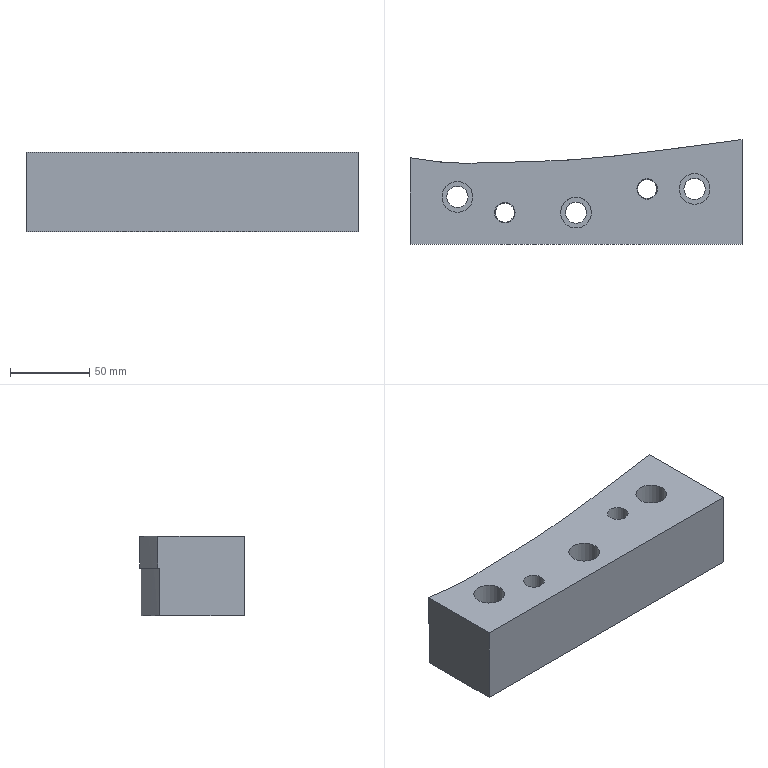Part | NX | features solid 2 | 1 solid | 23 faces | box 210 x 66.209 x 50 mm | volume 539295 mm3 | plane 11 | cylinder 10 | spline 2 | commonest cylinder face diameters 13.5 x3 19.5 x3 12 x2 13 x2
STEP:
#1=CARTESIAN_POINT('',(95.,106.209,-20.));
#2=VERTEX_POINT('',#1);
#3=CARTESIAN_POINT('',(95.,106.209,0.));
#4=VERTEX_POINT('',#3);
#5=CARTESIAN_POINT('',(95.,106.209,-10.));
#6=DIRECTION('',(0.,0.,-1.));
#7=VECTOR('',#6,1000.);
#8=LINE('',#5,#7);
#9=EDGE_CURVE('',#2,#4,#8,.F.);
#10=ORIENTED_EDGE('',*,*,#9,.F.);
#11=CARTESIAN_POINT('',(-115.,94.682,-20.));
#12=VERTEX_POINT('',#11);
#13=CARTESIAN_POINT('',(-190.231,-121.49,-20.));
#14=CARTESIAN_POINT('',(-188.654,-121.152,-20.));
#15=CARTESIAN_POINT('',(-185.47,-120.627,-20.));
#16=CARTESIAN_POINT('',(-180.656,-120.141,-20.));
#17=CARTESIAN_POINT('',(-175.882,-119.326,-20.));
#18=CARTESIAN_POINT('',(-169.679,-117.528,-20.));
#19=CARTESIAN_POINT('',(-162.185,-114.539,-20.));
#20=CARTESIAN_POINT('',(-153.086,-111.254,-20.));
#21=CARTESIAN_POINT('',(-144.031,-107.845,-20.));
#22=CARTESIAN_POINT('',(-136.465,-105.061,-20.));
#23=CARTESIAN_POINT('',(-130.418,-102.814,-20.));
#24=CARTESIAN_POINT('',(-125.812,-101.329,-20.));
#25=CARTESIAN_POINT('',(-121.306,-99.566,-20.));
#26=CARTESIAN_POINT('',(-116.876,-97.626,-20.));
#27=CARTESIAN_POINT('',(-112.335,-95.923,-20.));
#28=CARTESIAN_POINT('',(-107.564,-95.05,-20.));
#29=CARTESIAN_POINT('',(-102.756,-94.525,-20.));
#30=CARTESIAN_POINT('',(-96.349,-93.771,-20.));
#31=CARTESIAN_POINT('',(-89.902,-93.468,-20.));
#32=CARTESIAN_POINT('',(-83.452,-93.448,-20.));
#33=CARTESIAN_POINT('',(-77.002,-93.469,-20.));
#34=CARTESIAN_POINT('',(-68.939,-93.411,-20.));
#35=CARTESIAN_POINT('',(-56.04,-93.3,-20.));
#36=CARTESIAN_POINT('',(-33.465,-93.184,-20.));
#37=CARTESIAN_POINT('',(-7.666,-93.074,-20.));
#38=CARTESIAN_POINT('',(14.907,-92.653,-20.));
#39=CARTESIAN_POINT('',(27.794,-92.068,-20.));
#40=CARTESIAN_POINT('',(40.668,-91.245,-20.));
#41=CARTESIAN_POINT('',(51.917,-90.291,-20.));
#42=CARTESIAN_POINT('',(61.528,-89.174,-20.));
#43=CARTESIAN_POINT('',(67.939,-88.466,-20.));
#44=CARTESIAN_POINT('',(79.125,-86.95,-20.));
#45=CARTESIAN_POINT('',(95.161,-85.253,-20.));
#46=CARTESIAN_POINT('',(114.404,-83.21,-20.));
#47=CARTESIAN_POINT('',(133.568,-80.524,-20.));
#48=CARTESIAN_POINT('',(152.734,-77.861,-20.));
#49=CARTESIAN_POINT('',(171.916,-75.326,-20.));
#50=CARTESIAN_POINT('',(191.055,-72.413,-20.));
#51=CARTESIAN_POINT('',(207.17,-71.468,-20.));
#52=CARTESIAN_POINT('',(219.951,-69.697,-20.));
#53=CARTESIAN_POINT('',(232.724,-67.899,-20.));
#54=CARTESIAN_POINT('',(248.708,-65.766,-20.));
#55=CARTESIAN_POINT('',(267.87,-63.074,-20.));
#56=CARTESIAN_POINT('',(287.038,-60.44,-20.));
#57=CARTESIAN_POINT('',(301.448,-58.682,-20.));
#58=CARTESIAN_POINT('',(310.976,-56.987,-20.));
#59=CARTESIAN_POINT('',(314.916,-56.135,-20.));
#60=CARTESIAN_POINT('',(318.052,-55.382,-20.));
#61=CARTESIAN_POINT('',(320.39,-54.76,-20.));
#62=CARTESIAN_POINT('',(322.686,-53.981,-20.));
#63=CARTESIAN_POINT('',(325.595,-52.578,-20.));
#64=CARTESIAN_POINT('',(328.769,-50.098,-20.));
#65=CARTESIAN_POINT('',(332.247,-46.69,-20.));
#66=CARTESIAN_POINT('',(335.795,-43.406,-20.));
#67=CARTESIAN_POINT('',(343.661,-37.758,-20.));
#68=CARTESIAN_POINT('',(355.164,-28.914,-20.));
#69=CARTESIAN_POINT('',(370.422,-17.018,-20.));
#70=CARTESIAN_POINT('',(383.264,-7.249,-20.));
#71=CARTESIAN_POINT('',(392.416,-0.6713,-20.));
#72=CARTESIAN_POINT('',(396.953,2.733,-20.));
#73=CARTESIAN_POINT('',(398.886,5.372,-20.));
#74=CARTESIAN_POINT('',(399.725,7.654,-20.));
#75=CARTESIAN_POINT('',(399.76,10.078,-20.));
#76=CARTESIAN_POINT('',(399.483,13.317,-20.));
#77=CARTESIAN_POINT('',(399.712,17.34,-20.));
#78=CARTESIAN_POINT('',(399.612,22.179,-20.));
#79=CARTESIAN_POINT('',(399.633,31.854,-20.));
#80=CARTESIAN_POINT('',(399.593,46.366,-20.));
#81=CARTESIAN_POINT('',(399.637,62.491,-20.));
#82=CARTESIAN_POINT('',(399.588,73.779,-20.));
#83=CARTESIAN_POINT('',(399.652,79.422,-20.));
#84=CARTESIAN_POINT('',(399.59,82.647,-20.));
#85=CARTESIAN_POINT('',(399.564,85.065,-20.));
#86=CARTESIAN_POINT('',(399.725,87.486,-20.));
#87=CARTESIAN_POINT('',(399.756,89.902,-20.));
#88=CARTESIAN_POINT('',(399.247,92.301,-20.));
#89=CARTESIAN_POINT('',(397.362,95.008,-20.));
#90=CARTESIAN_POINT('',(393.635,96.774,-20.));
#91=CARTESIAN_POINT('',(389.279,98.826,-20.));
#92=CARTESIAN_POINT('',(384.732,100.498,-20.));
#93=CARTESIAN_POINT('',(378.765,102.95,-20.));
#94=CARTESIAN_POINT('',(362.589,110.229,-20.));
#95=CARTESIAN_POINT('',(344.928,118.135,-20.));
#96=CARTESIAN_POINT('',(327.281,126.072,-20.));
#97=CARTESIAN_POINT('',(319.932,129.381,-20.));
#98=CARTESIAN_POINT('',(314.075,132.102,-20.));
#99=CARTESIAN_POINT('',(309.387,133.376,-20.));
#100=CARTESIAN_POINT('',(304.547,133.785,-20.));
#101=CARTESIAN_POINT('',(299.716,133.401,-20.));
#102=CARTESIAN_POINT('',(294.929,132.704,-20.));
#103=CARTESIAN_POINT('',(288.543,131.8,-20.));
#104=CARTESIAN_POINT('',(277.364,130.241,-20.));
#105=CARTESIAN_POINT('',(242.2,125.552,-20.));
#106=CARTESIAN_POINT('',(184.637,118.048,-20.));
#107=CARTESIAN_POINT('',(120.701,109.541,-20.));
#108=CARTESIAN_POINT('',(69.531,102.902,-20.));
#109=CARTESIAN_POINT('',(40.777,98.94,-20.));
#110=CARTESIAN_POINT('',(21.566,96.615,-20.));
#111=CARTESIAN_POINT('',(8.743,95.212,-20.));
#112=CARTESIAN_POINT('',(-7.301,93.575,-20.));
#113=CARTESIAN_POINT('',(-26.625,92.505,-20.));
#114=CARTESIAN_POINT('',(-45.971,92.017,-20.));
#115=CARTESIAN_POINT('',(-62.09,91.675,-20.));
#116=CARTESIAN_POINT('',(-74.987,91.256,-20.));
#117=CARTESIAN_POINT('',(-84.664,91.165,-20.));
#118=CARTESIAN_POINT('',(-94.319,91.781,-20.));
#119=CARTESIAN_POINT('',(-103.929,92.966,-20.));
#120=CARTESIAN_POINT('',(-113.495,94.403,-20.));
#121=CARTESIAN_POINT('',(-119.856,95.492,-20.));
#122=CARTESIAN_POINT('',(-122.997,96.222,-20.));
#123=B_SPLINE_CURVE_WITH_KNOTS('',3,(#13,#14,#15,#16,#17,#18,#19,#20,#21,#22,#23,#24,#25,#26,#27,#28,#29,#30,#31,#32,#33,#34,#35,#36,#37,#38,#39,#40,#41,#42,#43,#44,#45,#46,#47,#48,#49,#50,#51,#52,#53,#54,#55,#56,#57,#58,#59,#60,#61,#62,#63,#64,#65,#66,#67,#68,#69,#70,#71,#72,#73,#74,#75,#76,#77,#78,#79,#80,#81,#82,#83,#84,#85,#86,#87,#88,#89,#90,#91,#92,#93,#94,#95,#96,#97,#98,#99,#100,#101,#102,#103,#104,#105,#106,#107,#108,#109,#110,#111,#112,#113,#114,#115,#116,#117,#118,#119,#120,#121,#122),.UNSPECIFIED.,.F.,.F.,(4,1,1,1,1,1,1,1,1,1,1,1,1,1,1,1,1,1,1,1,1,1,1,1,1,1,1,1,1,1,1,1,1,1,1,1,1,1,1,1,1,1,1,1,1,1,1,1,1,1,1,1,1,1,1,1,1,1,1,1,1,1,1,1,1,1,1,1,1,1,1,1,1,1,1,1,1,1,1,1,1,1,1,1,1,1,1,1,1,1,1,1,1,1,1,1,1,1,1,1,1,1,1,1,1,1,1,4),(0.4704,0.4724,0.4745,0.4766,0.4786,0.4828,0.4869,0.491,0.4952,0.4972,0.4993,0.5014,0.5035,0.5055,0.5076,0.5097,0.5117,0.5159,0.5179,0.52,0.5241,0.5283,0.5366,0.5531,0.5614,0.5655,0.5697,0.5779,0.58,0.5821,0.5862,0.5945,0.6028,0.611,0.6193,0.6276,0.6359,0.6441,0.6483,0.6524,0.6607,0.669,0.6772,0.6855,0.6876,0.6897,0.6907,0.6917,0.6928,0.6938,0.6959,0.6979,0.7,0.7021,0.7103,0.7186,0.7269,0.731,0.7331,0.7341,0.7352,0.7362,0.7372,0.7393,0.7414,0.7435,0.7517,0.76,0.7641,0.7662,0.7672,0.7683,0.7693,0.7703,0.7714,0.7724,0.7745,0.7766,0.7786,0.7807,0.7848,0.8014,0.8055,0.8097,0.8117,0.8138,0.8159,0.8179,0.82,0.8221,0.8262,0.8345,0.8676,0.9007,0.9172,0.9338,0.9379,0.9421,0.9503,0.9586,0.9669,0.9752,0.9793,0.9834,0.9876,0.9917,0.9959,1.),.UNSPECIFIED.);
#124=EDGE_CURVE('',#2,#12,#123,.T.);
#125=ORIENTED_EDGE('',*,*,#124,.T.);
#126=CARTESIAN_POINT('',(-115.,94.682,0.));
#127=VERTEX_POINT('',#126);
#128=CARTESIAN_POINT('',(-115.,94.682,-35.));
#129=DIRECTION('',(0.,0.,-1.));
#130=VECTOR('',#129,1000.);
#131=LINE('',#128,#130);
#132=EDGE_CURVE('',#12,#127,#131,.F.);
#133=ORIENTED_EDGE('',*,*,#132,.T.);
#134=CARTESIAN_POINT('',(-115.,94.682,0.));
#135=CARTESIAN_POINT('',(-110.608,93.956,0.));
#136=CARTESIAN_POINT('',(-101.827,92.632,0.));
#137=CARTESIAN_POINT('',(-84.275,90.758,0.));
#138=CARTESIAN_POINT('',(-62.384,91.781,0.));
#139=CARTESIAN_POINT('',(-36.103,92.158,0.));
#140=CARTESIAN_POINT('',(-9.834,93.269,0.));
#141=CARTESIAN_POINT('',(16.416,95.966,0.));
#142=CARTESIAN_POINT('',(42.64,99.193,0.));
#143=CARTESIAN_POINT('',(68.808,102.78,0.));
#144=CARTESIAN_POINT('',(86.269,105.068,0.));
#145=CARTESIAN_POINT('',(95.,106.209,0.));
#146=B_SPLINE_CURVE_WITH_KNOTS('',3,(#134,#135,#136,#137,#138,#139,#140,#141,#142,#143,#144,#145),.UNSPECIFIED.,.F.,.F.,(4,1,1,1,1,1,1,1,1,4),(0.,0.01314,0.02628,0.05257,0.07885,0.1051,0.1314,0.1577,0.184,0.2103),.UNSPECIFIED.);
#147=EDGE_CURVE('',#127,#4,#146,.T.);
#148=ORIENTED_EDGE('',*,*,#147,.T.);
#149=EDGE_LOOP('',(#10,#125,#133,#148));
#150=FACE_BOUND('',#149,.T.);
#151=CARTESIAN_POINT('',(95.,106.209,0.));
#152=CARTESIAN_POINT('',(95.,106.209,-20.));
#153=CARTESIAN_POINT('',(86.281,105.069,0.));
#154=CARTESIAN_POINT('',(86.281,105.069,-20.));
#155=CARTESIAN_POINT('',(68.844,102.785,0.));
#156=CARTESIAN_POINT('',(68.844,102.785,-20.));
#157=CARTESIAN_POINT('',(42.708,99.202,0.));
#158=CARTESIAN_POINT('',(42.708,99.202,-20.));
#159=CARTESIAN_POINT('',(16.527,95.979,0.));
#160=CARTESIAN_POINT('',(16.527,95.979,-20.));
#161=CARTESIAN_POINT('',(-9.721,93.276,0.));
#162=CARTESIAN_POINT('',(-9.721,93.276,-20.));
#163=CARTESIAN_POINT('',(-36.089,92.158,0.));
#164=CARTESIAN_POINT('',(-36.089,92.158,-20.));
#165=CARTESIAN_POINT('',(-62.452,91.777,0.));
#166=CARTESIAN_POINT('',(-62.452,91.777,-20.));
#167=CARTESIAN_POINT('',(-84.459,90.762,0.));
#168=CARTESIAN_POINT('',(-84.459,90.762,-20.));
#169=CARTESIAN_POINT('',(-101.968,92.654,0.));
#170=CARTESIAN_POINT('',(-101.968,92.654,-20.));
#171=CARTESIAN_POINT('',(-110.662,93.965,0.));
#172=CARTESIAN_POINT('',(-110.662,93.965,-20.));
#173=CARTESIAN_POINT('',(-115.,94.682,0.));
#174=CARTESIAN_POINT('',(-115.,94.682,-20.));
#175=B_SPLINE_SURFACE_WITH_KNOTS('',3,1,((#151,#152),(#153,#154),(#155,#156),(#157,#158),(#159,#160),(#161,#162),(#163,#164),(#165,#166),(#167,#168),(#169,#170),(#171,#172),(#173,#174)),.SURF_OF_LINEAR_EXTRUSION.,.F.,.F.,.F.,(4,1,1,1,1,1,1,1,1,4),(2,2),(0.9063,0.9175,0.9288,0.9401,0.9514,0.9627,0.974,0.9852,0.9909,0.9965),(0.,1.),.UNSPECIFIED.);
#176=ADVANCED_FACE('',(#150),#175,.F.);
#177=CARTESIAN_POINT('',(95.,105.2,-20.));
#178=VERTEX_POINT('',#177);
#179=CARTESIAN_POINT('',(95.,83.097,-20.));
#180=DIRECTION('',(0.,-1.,0.));
#181=VECTOR('',#180,1000.);
#182=LINE('',#179,#181);
#183=EDGE_CURVE('',#2,#178,#182,.T.);
#184=ORIENTED_EDGE('',*,*,#183,.F.);
#185=ORIENTED_EDGE('',*,*,#9,.T.);
#186=CARTESIAN_POINT('',(95.,40.,0.));
#187=VERTEX_POINT('',#186);
#188=CARTESIAN_POINT('',(95.,-222.,0.));
#189=DIRECTION('',(0.,-1.,0.));
#190=VECTOR('',#189,1000.);
#191=LINE('',#188,#190);
#192=EDGE_CURVE('',#4,#187,#191,.T.);
#193=ORIENTED_EDGE('',*,*,#192,.T.);
#194=CARTESIAN_POINT('',(95.,40.,-50.));
#195=VERTEX_POINT('',#194);
#196=CARTESIAN_POINT('',(95.,40.,0.));
#197=DIRECTION('',(0.,0.,-1.));
#198=VECTOR('',#197,1000.);
#199=LINE('',#196,#198);
#200=EDGE_CURVE('',#187,#195,#199,.T.);
#201=ORIENTED_EDGE('',*,*,#200,.T.);
#202=CARTESIAN_POINT('',(95.,105.2,-50.));
#203=VERTEX_POINT('',#202);
#204=CARTESIAN_POINT('',(95.,35.09,-50.));
#205=DIRECTION('',(0.,1.,0.));
#206=VECTOR('',#205,1000.);
#207=LINE('',#204,#206);
#208=EDGE_CURVE('',#195,#203,#207,.T.);
#209=ORIENTED_EDGE('',*,*,#208,.T.);
#210=CARTESIAN_POINT('',(95.,105.2,-60.));
#211=DIRECTION('',(0.,0.,-1.));
#212=VECTOR('',#211,1000.);
#213=LINE('',#210,#212);
#214=EDGE_CURVE('',#178,#203,#213,.T.);
#215=ORIENTED_EDGE('',*,*,#214,.F.);
#216=EDGE_LOOP('',(#184,#185,#193,#201,#209,#215));
#217=FACE_BOUND('',#216,.T.);
#218=CARTESIAN_POINT('',(95.,83.097,-25.));
#219=DIRECTION('',(1.,0.,0.));
#220=DIRECTION('',(0.,0.,-1.));
#221=AXIS2_PLACEMENT_3D('',#218,#219,#220);
#222=PLANE('',#221);
#223=ADVANCED_FACE('',(#217),#222,.T.);
#224=ORIENTED_EDGE('',*,*,#132,.F.);
#225=CARTESIAN_POINT('',(-115.,93.668,-20.));
#226=VERTEX_POINT('',#225);
#227=CARTESIAN_POINT('',(-115.,30.,-20.));
#228=DIRECTION('',(0.,-1.,0.));
#229=VECTOR('',#228,1000.);
#230=LINE('',#227,#229);
#231=EDGE_CURVE('',#12,#226,#230,.T.);
#232=ORIENTED_EDGE('',*,*,#231,.T.);
#233=CARTESIAN_POINT('',(-115.,93.668,-50.));
#234=VERTEX_POINT('',#233);
#235=CARTESIAN_POINT('',(-115.,93.668,-60.));
#236=DIRECTION('',(0.,0.,-1.));
#237=VECTOR('',#236,1000.);
#238=LINE('',#235,#237);
#239=EDGE_CURVE('',#226,#234,#238,.T.);
#240=ORIENTED_EDGE('',*,*,#239,.T.);
#241=CARTESIAN_POINT('',(-115.,40.,-50.));
#242=VERTEX_POINT('',#241);
#243=CARTESIAN_POINT('',(-115.,35.09,-50.));
#244=DIRECTION('',(0.,1.,0.));
#245=VECTOR('',#244,1000.);
#246=LINE('',#243,#245);
#247=EDGE_CURVE('',#242,#234,#246,.T.);
#248=ORIENTED_EDGE('',*,*,#247,.F.);
#249=CARTESIAN_POINT('',(-115.,40.,0.));
#250=VERTEX_POINT('',#249);
#251=CARTESIAN_POINT('',(-115.,40.,0.));
#252=DIRECTION('',(0.,0.,1.));
#253=VECTOR('',#252,1000.);
#254=LINE('',#251,#253);
#255=EDGE_CURVE('',#242,#250,#254,.T.);
#256=ORIENTED_EDGE('',*,*,#255,.T.);
#257=CARTESIAN_POINT('',(-115.,-222.,0.));
#258=DIRECTION('',(0.,-1.,0.));
#259=VECTOR('',#258,1000.);
#260=LINE('',#257,#259);
#261=EDGE_CURVE('',#127,#250,#260,.T.);
#262=ORIENTED_EDGE('',*,*,#261,.F.);
#263=EDGE_LOOP('',(#224,#232,#240,#248,#256,#262));
#264=FACE_BOUND('',#263,.T.);
#265=CARTESIAN_POINT('',(-115.,30.,0.));
#266=DIRECTION('',(1.,0.,0.));
#267=DIRECTION('',(0.,0.,-1.));
#268=AXIS2_PLACEMENT_3D('',#265,#266,#267);
#269=PLANE('',#268);
#270=ADVANCED_FACE('',(#264),#269,.F.);
#271=ORIENTED_EDGE('',*,*,#200,.F.);
#272=CARTESIAN_POINT('',(-470.381,40.,0.));
#273=DIRECTION('',(1.,0.,0.));
#274=VECTOR('',#273,1000.);
#275=LINE('',#272,#274);
#276=EDGE_CURVE('',#250,#187,#275,.T.);
#277=ORIENTED_EDGE('',*,*,#276,.F.);
#278=ORIENTED_EDGE('',*,*,#255,.F.);
#279=CARTESIAN_POINT('',(-415.478,40.,-50.));
#280=DIRECTION('',(-1.,0.,0.));
#281=VECTOR('',#280,1000.);
#282=LINE('',#279,#281);
#283=EDGE_CURVE('',#195,#242,#282,.T.);
#284=ORIENTED_EDGE('',*,*,#283,.F.);
#285=EDGE_LOOP('',(#271,#277,#278,#284));
#286=FACE_BOUND('',#285,.T.);
#287=CARTESIAN_POINT('',(180.,40.,0.));
#288=DIRECTION('',(0.,1.,0.));
#289=DIRECTION('',(0.,0.,1.));
#290=AXIS2_PLACEMENT_3D('',#287,#288,#289);
#291=PLANE('',#290);
#292=ADVANCED_FACE('',(#286),#291,.F.);
#293=CARTESIAN_POINT('',(28.5,75.,0.));
#294=VERTEX_POINT('',#293);
#295=CARTESIAN_POINT('',(35.,75.,0.));
#296=DIRECTION('',(0.,0.,-1.));
#297=DIRECTION('',(-1.,0.,0.));
#298=AXIS2_PLACEMENT_3D('',#295,#296,#297);
#299=CIRCLE('',#298,6.5);
#300=EDGE_CURVE('',#294,#294,#299,.T.);
#301=ORIENTED_EDGE('',*,*,#300,.T.);
#302=EDGE_LOOP('',(#301));
#303=FACE_BOUND('',#302,.T.);
#304=CARTESIAN_POINT('',(-61.5,60.,0.));
#305=VERTEX_POINT('',#304);
#306=CARTESIAN_POINT('',(-55.,60.,0.));
#307=DIRECTION('',(0.,0.,-1.));
#308=DIRECTION('',(-1.,0.,0.));
#309=AXIS2_PLACEMENT_3D('',#306,#307,#308);
#310=CIRCLE('',#309,6.5);
#311=EDGE_CURVE('',#305,#305,#310,.T.);
#312=ORIENTED_EDGE('',*,*,#311,.T.);
#313=EDGE_LOOP('',(#312));
#314=FACE_BOUND('',#313,.T.);
#315=CARTESIAN_POINT('',(-19.75,60.,0.));
#316=VERTEX_POINT('',#315);
#317=CARTESIAN_POINT('',(-10.,60.,0.));
#318=DIRECTION('',(0.,0.,-1.));
#319=DIRECTION('',(-1.,0.,0.));
#320=AXIS2_PLACEMENT_3D('',#317,#318,#319);
#321=CIRCLE('',#320,9.75);
#322=EDGE_CURVE('',#316,#316,#321,.T.);
#323=ORIENTED_EDGE('',*,*,#322,.T.);
#324=EDGE_LOOP('',(#323));
#325=FACE_BOUND('',#324,.T.);
#326=CARTESIAN_POINT('',(55.25,75.,0.));
#327=VERTEX_POINT('',#326);
#328=CARTESIAN_POINT('',(65.,75.,0.));
#329=DIRECTION('',(0.,0.,-1.));
#330=DIRECTION('',(-1.,0.,0.));
#331=AXIS2_PLACEMENT_3D('',#328,#329,#330);
#332=CIRCLE('',#331,9.75);
#333=EDGE_CURVE('',#327,#327,#332,.T.);
#334=ORIENTED_EDGE('',*,*,#333,.T.);
#335=EDGE_LOOP('',(#334));
#336=FACE_BOUND('',#335,.T.);
#337=CARTESIAN_POINT('',(-94.75,70.,0.));
#338=VERTEX_POINT('',#337);
#339=CARTESIAN_POINT('',(-85.,70.,0.));
#340=DIRECTION('',(0.,0.,-1.));
#341=DIRECTION('',(-1.,0.,0.));
#342=AXIS2_PLACEMENT_3D('',#339,#340,#341);
#343=CIRCLE('',#342,9.75);
#344=EDGE_CURVE('',#338,#338,#343,.T.);
#345=ORIENTED_EDGE('',*,*,#344,.T.);
#346=EDGE_LOOP('',(#345));
#347=FACE_BOUND('',#346,.T.);
#348=ORIENTED_EDGE('',*,*,#192,.F.);
#349=ORIENTED_EDGE('',*,*,#147,.F.);
#350=ORIENTED_EDGE('',*,*,#261,.T.);
#351=ORIENTED_EDGE('',*,*,#276,.T.);
#352=EDGE_LOOP('',(#348,#349,#350,#351));
#353=FACE_BOUND('',#352,.T.);
#354=CARTESIAN_POINT('',(-470.381,-222.,0.));
#355=DIRECTION('',(0.,0.,-1.));
#356=DIRECTION('',(-1.,0.,0.));
#357=AXIS2_PLACEMENT_3D('',#354,#355,#356);
#358=PLANE('',#357);
#359=ADVANCED_FACE('',(#303,#314,#325,#336,#347,#353),#358,.F.);
#360=CARTESIAN_POINT('',(41.,75.,-50.));
#361=VERTEX_POINT('',#360);
#362=CARTESIAN_POINT('',(35.,75.,-50.));
#363=DIRECTION('',(0.,0.,1.));
#364=DIRECTION('',(1.,0.,0.));
#365=AXIS2_PLACEMENT_3D('',#362,#363,#364);
#366=CIRCLE('',#365,6.);
#367=EDGE_CURVE('',#361,#361,#366,.T.);
#368=ORIENTED_EDGE('',*,*,#367,.T.);
#369=EDGE_LOOP('',(#368));
#370=FACE_BOUND('',#369,.T.);
#371=CARTESIAN_POINT('',(-49.,60.,-50.));
#372=VERTEX_POINT('',#371);
#373=CARTESIAN_POINT('',(-55.,60.,-50.));
#374=DIRECTION('',(0.,0.,1.));
#375=DIRECTION('',(1.,0.,0.));
#376=AXIS2_PLACEMENT_3D('',#373,#374,#375);
#377=CIRCLE('',#376,6.);
#378=EDGE_CURVE('',#372,#372,#377,.T.);
#379=ORIENTED_EDGE('',*,*,#378,.T.);
#380=EDGE_LOOP('',(#379));
#381=FACE_BOUND('',#380,.T.);
#382=CARTESIAN_POINT('',(-3.25,60.,-50.));
#383=VERTEX_POINT('',#382);
#384=CARTESIAN_POINT('',(-10.,60.,-50.));
#385=DIRECTION('',(0.,0.,1.));
#386=DIRECTION('',(1.,0.,0.));
#387=AXIS2_PLACEMENT_3D('',#384,#385,#386);
#388=CIRCLE('',#387,6.75);
#389=EDGE_CURVE('',#383,#383,#388,.T.);
#390=ORIENTED_EDGE('',*,*,#389,.T.);
#391=EDGE_LOOP('',(#390));
#392=FACE_BOUND('',#391,.T.);
#393=CARTESIAN_POINT('',(71.75,75.,-50.));
#394=VERTEX_POINT('',#393);
#395=CARTESIAN_POINT('',(65.,75.,-50.));
#396=DIRECTION('',(0.,0.,1.));
#397=DIRECTION('',(1.,0.,0.));
#398=AXIS2_PLACEMENT_3D('',#395,#396,#397);
#399=CIRCLE('',#398,6.75);
#400=EDGE_CURVE('',#394,#394,#399,.T.);
#401=ORIENTED_EDGE('',*,*,#400,.T.);
#402=EDGE_LOOP('',(#401));
#403=FACE_BOUND('',#402,.T.);
#404=CARTESIAN_POINT('',(-78.25,70.,-50.));
#405=VERTEX_POINT('',#404);
#406=CARTESIAN_POINT('',(-85.,70.,-50.));
#407=DIRECTION('',(0.,0.,1.));
#408=DIRECTION('',(1.,0.,0.));
#409=AXIS2_PLACEMENT_3D('',#406,#407,#408);
#410=CIRCLE('',#409,6.75);
#411=EDGE_CURVE('',#405,#405,#410,.T.);
#412=ORIENTED_EDGE('',*,*,#411,.T.);
#413=EDGE_LOOP('',(#412));
#414=FACE_BOUND('',#413,.T.);
#415=ORIENTED_EDGE('',*,*,#247,.T.);
#416=CARTESIAN_POINT('',(-115.,93.668,-50.));
#417=CARTESIAN_POINT('',(-110.605,92.944,-50.));
#418=CARTESIAN_POINT('',(-101.817,91.621,-50.));
#419=CARTESIAN_POINT('',(-84.257,89.76,-50.));
#420=CARTESIAN_POINT('',(-62.371,90.78,-50.));
#421=CARTESIAN_POINT('',(-36.092,91.159,-50.));
#422=CARTESIAN_POINT('',(-9.827,92.267,-50.));
#423=CARTESIAN_POINT('',(16.408,94.959,-50.));
#424=CARTESIAN_POINT('',(42.632,98.183,-50.));
#425=CARTESIAN_POINT('',(68.805,101.771,-50.));
#426=CARTESIAN_POINT('',(86.268,104.059,-50.));
#427=CARTESIAN_POINT('',(95.,105.2,-50.));
#428=B_SPLINE_CURVE_WITH_KNOTS('',3,(#416,#417,#418,#419,#420,#421,#422,#423,#424,#425,#426,#427),.UNSPECIFIED.,.F.,.F.,(4,1,1,1,1,1,1,1,1,4),(0.,0.01314,0.02628,0.05256,0.07884,0.1051,0.1314,0.1577,0.184,0.2103),.UNSPECIFIED.);
#429=EDGE_CURVE('',#234,#203,#428,.T.);
#430=ORIENTED_EDGE('',*,*,#429,.T.);
#431=ORIENTED_EDGE('',*,*,#208,.F.);
#432=ORIENTED_EDGE('',*,*,#283,.T.);
#433=EDGE_LOOP('',(#415,#430,#431,#432));
#434=FACE_BOUND('',#433,.T.);
#435=CARTESIAN_POINT('',(-415.478,35.09,-50.));
#436=DIRECTION('',(0.,0.,1.));
#437=DIRECTION('',(1.,0.,0.));
#438=AXIS2_PLACEMENT_3D('',#435,#436,#437);
#439=PLANE('',#438);
#440=ADVANCED_FACE('',(#370,#381,#392,#403,#414,#434),#439,.F.);
#441=CARTESIAN_POINT('',(-91.75,70.,-15.));
#442=VERTEX_POINT('',#441);
#443=CARTESIAN_POINT('',(-85.,70.,-15.));
#444=DIRECTION('',(0.,0.,-1.));
#445=DIRECTION('',(-1.,0.,0.));
#446=AXIS2_PLACEMENT_3D('',#443,#444,#445);
#447=CIRCLE('',#446,6.75);
#448=EDGE_CURVE('',#442,#442,#447,.T.);
#449=ORIENTED_EDGE('',*,*,#448,.F.);
#450=EDGE_LOOP('',(#449));
#451=FACE_BOUND('',#450,.T.);
#452=ORIENTED_EDGE('',*,*,#411,.F.);
#453=EDGE_LOOP('',(#452));
#454=FACE_BOUND('',#453,.T.);
#455=CARTESIAN_POINT('',(-85.,70.,-100.));
#456=DIRECTION('',(0.,0.,-1.));
#457=DIRECTION('',(-1.,0.,0.));
#458=AXIS2_PLACEMENT_3D('',#455,#456,#457);
#459=CYLINDRICAL_SURFACE('',#458,6.75);
#460=ADVANCED_FACE('',(#451,#454),#459,.F.);
#461=ORIENTED_EDGE('',*,*,#448,.T.);
#462=EDGE_LOOP('',(#461));
#463=FACE_BOUND('',#462,.T.);
#464=CARTESIAN_POINT('',(-94.75,70.,-15.));
#465=VERTEX_POINT('',#464);
#466=CARTESIAN_POINT('',(-85.,70.,-15.));
#467=DIRECTION('',(0.,0.,-1.));
#468=DIRECTION('',(-1.,0.,0.));
#469=AXIS2_PLACEMENT_3D('',#466,#467,#468);
#470=CIRCLE('',#469,9.75);
#471=EDGE_CURVE('',#465,#465,#470,.T.);
#472=ORIENTED_EDGE('',*,*,#471,.F.);
#473=EDGE_LOOP('',(#472));
#474=FACE_BOUND('',#473,.T.);
#475=CARTESIAN_POINT('',(-85.,65.,-15.));
#476=DIRECTION('',(0.,0.,-1.));
#477=DIRECTION('',(-1.,0.,0.));
#478=AXIS2_PLACEMENT_3D('',#475,#476,#477);
#479=PLANE('',#478);
#480=ADVANCED_FACE('',(#463,#474),#479,.F.);
#481=ORIENTED_EDGE('',*,*,#471,.T.);
#482=EDGE_LOOP('',(#481));
#483=FACE_BOUND('',#482,.T.);
#484=ORIENTED_EDGE('',*,*,#344,.F.);
#485=EDGE_LOOP('',(#484));
#486=FACE_BOUND('',#485,.T.);
#487=CARTESIAN_POINT('',(-85.,70.,0.));
#488=DIRECTION('',(0.,0.,-1.));
#489=DIRECTION('',(-1.,0.,0.));
#490=AXIS2_PLACEMENT_3D('',#487,#488,#489);
#491=CYLINDRICAL_SURFACE('',#490,9.75);
#492=ADVANCED_FACE('',(#483,#486),#491,.F.);
#493=CARTESIAN_POINT('',(58.25,75.,-15.));
#494=VERTEX_POINT('',#493);
#495=CARTESIAN_POINT('',(65.,75.,-15.));
#496=DIRECTION('',(0.,0.,-1.));
#497=DIRECTION('',(-1.,0.,0.));
#498=AXIS2_PLACEMENT_3D('',#495,#496,#497);
#499=CIRCLE('',#498,6.75);
#500=EDGE_CURVE('',#494,#494,#499,.T.);
#501=ORIENTED_EDGE('',*,*,#500,.F.);
#502=EDGE_LOOP('',(#501));
#503=FACE_BOUND('',#502,.T.);
#504=ORIENTED_EDGE('',*,*,#400,.F.);
#505=EDGE_LOOP('',(#504));
#506=FACE_BOUND('',#505,.T.);
#507=CARTESIAN_POINT('',(65.,75.,-100.));
#508=DIRECTION('',(0.,0.,-1.));
#509=DIRECTION('',(-1.,0.,0.));
#510=AXIS2_PLACEMENT_3D('',#507,#508,#509);
#511=CYLINDRICAL_SURFACE('',#510,6.75);
#512=ADVANCED_FACE('',(#503,#506),#511,.F.);
#513=ORIENTED_EDGE('',*,*,#500,.T.);
#514=EDGE_LOOP('',(#513));
#515=FACE_BOUND('',#514,.T.);
#516=CARTESIAN_POINT('',(55.25,75.,-15.));
#517=VERTEX_POINT('',#516);
#518=CARTESIAN_POINT('',(65.,75.,-15.));
#519=DIRECTION('',(0.,0.,-1.));
#520=DIRECTION('',(-1.,0.,0.));
#521=AXIS2_PLACEMENT_3D('',#518,#519,#520);
#522=CIRCLE('',#521,9.75);
#523=EDGE_CURVE('',#517,#517,#522,.T.);
#524=ORIENTED_EDGE('',*,*,#523,.F.);
#525=EDGE_LOOP('',(#524));
#526=FACE_BOUND('',#525,.T.);
#527=CARTESIAN_POINT('',(65.,75.,-15.));
#528=DIRECTION('',(0.,0.,-1.));
#529=DIRECTION('',(-1.,0.,0.));
#530=AXIS2_PLACEMENT_3D('',#527,#528,#529);
#531=PLANE('',#530);
#532=ADVANCED_FACE('',(#515,#526),#531,.F.);
#533=ORIENTED_EDGE('',*,*,#523,.T.);
#534=EDGE_LOOP('',(#533));
#535=FACE_BOUND('',#534,.T.);
#536=ORIENTED_EDGE('',*,*,#333,.F.);
#537=EDGE_LOOP('',(#536));
#538=FACE_BOUND('',#537,.T.);
#539=CARTESIAN_POINT('',(65.,75.,0.));
#540=DIRECTION('',(0.,0.,-1.));
#541=DIRECTION('',(-1.,0.,0.));
#542=AXIS2_PLACEMENT_3D('',#539,#540,#541);
#543=CYLINDRICAL_SURFACE('',#542,9.75);
#544=ADVANCED_FACE('',(#535,#538),#543,.F.);
#545=CARTESIAN_POINT('',(-16.75,60.,-15.));
#546=VERTEX_POINT('',#545);
#547=CARTESIAN_POINT('',(-10.,60.,-15.));
#548=DIRECTION('',(0.,0.,-1.));
#549=DIRECTION('',(-1.,0.,0.));
#550=AXIS2_PLACEMENT_3D('',#547,#548,#549);
#551=CIRCLE('',#550,6.75);
#552=EDGE_CURVE('',#546,#546,#551,.T.);
#553=ORIENTED_EDGE('',*,*,#552,.F.);
#554=EDGE_LOOP('',(#553));
#555=FACE_BOUND('',#554,.T.);
#556=ORIENTED_EDGE('',*,*,#389,.F.);
#557=EDGE_LOOP('',(#556));
#558=FACE_BOUND('',#557,.T.);
#559=CARTESIAN_POINT('',(-10.,60.,-100.));
#560=DIRECTION('',(0.,0.,-1.));
#561=DIRECTION('',(-1.,0.,0.));
#562=AXIS2_PLACEMENT_3D('',#559,#560,#561);
#563=CYLINDRICAL_SURFACE('',#562,6.75);
#564=ADVANCED_FACE('',(#555,#558),#563,.F.);
#565=ORIENTED_EDGE('',*,*,#552,.T.);
#566=EDGE_LOOP('',(#565));
#567=FACE_BOUND('',#566,.T.);
#568=CARTESIAN_POINT('',(-19.75,60.,-15.));
#569=VERTEX_POINT('',#568);
#570=CARTESIAN_POINT('',(-10.,60.,-15.));
#571=DIRECTION('',(0.,0.,-1.));
#572=DIRECTION('',(-1.,0.,0.));
#573=AXIS2_PLACEMENT_3D('',#570,#571,#572);
#574=CIRCLE('',#573,9.75);
#575=EDGE_CURVE('',#569,#569,#574,.T.);
#576=ORIENTED_EDGE('',*,*,#575,.F.);
#577=EDGE_LOOP('',(#576));
#578=FACE_BOUND('',#577,.T.);
#579=CARTESIAN_POINT('',(-10.,60.,-15.));
#580=DIRECTION('',(0.,0.,-1.));
#581=DIRECTION('',(-1.,0.,0.));
#582=AXIS2_PLACEMENT_3D('',#579,#580,#581);
#583=PLANE('',#582);
#584=ADVANCED_FACE('',(#567,#578),#583,.F.);
#585=ORIENTED_EDGE('',*,*,#575,.T.);
#586=EDGE_LOOP('',(#585));
#587=FACE_BOUND('',#586,.T.);
#588=ORIENTED_EDGE('',*,*,#322,.F.);
#589=EDGE_LOOP('',(#588));
#590=FACE_BOUND('',#589,.T.);
#591=CARTESIAN_POINT('',(-10.,60.,0.));
#592=DIRECTION('',(0.,0.,-1.));
#593=DIRECTION('',(-1.,0.,0.));
#594=AXIS2_PLACEMENT_3D('',#591,#592,#593);
#595=CYLINDRICAL_SURFACE('',#594,9.75);
#596=ADVANCED_FACE('',(#587,#590),#595,.F.);
#597=CARTESIAN_POINT('',(-61.,60.,-20.));
#598=VERTEX_POINT('',#597);
#599=CARTESIAN_POINT('',(-55.,60.,-20.));
#600=DIRECTION('',(0.,0.,-1.));
#601=DIRECTION('',(-1.,0.,0.));
#602=AXIS2_PLACEMENT_3D('',#599,#600,#601);
#603=CIRCLE('',#602,6.);
#604=EDGE_CURVE('',#598,#598,#603,.T.);
#605=ORIENTED_EDGE('',*,*,#604,.F.);
#606=EDGE_LOOP('',(#605));
#607=FACE_BOUND('',#606,.T.);
#608=ORIENTED_EDGE('',*,*,#378,.F.);
#609=EDGE_LOOP('',(#608));
#610=FACE_BOUND('',#609,.T.);
#611=CARTESIAN_POINT('',(-55.,60.,-100.));
#612=DIRECTION('',(0.,0.,-1.));
#613=DIRECTION('',(-1.,0.,0.));
#614=AXIS2_PLACEMENT_3D('',#611,#612,#613);
#615=CYLINDRICAL_SURFACE('',#614,6.);
#616=ADVANCED_FACE('',(#607,#610),#615,.F.);
#617=ORIENTED_EDGE('',*,*,#604,.T.);
#618=EDGE_LOOP('',(#617));
#619=FACE_BOUND('',#618,.T.);
#620=CARTESIAN_POINT('',(-61.5,60.,-20.));
#621=VERTEX_POINT('',#620);
#622=CARTESIAN_POINT('',(-55.,60.,-20.));
#623=DIRECTION('',(0.,0.,-1.));
#624=DIRECTION('',(-1.,0.,0.));
#625=AXIS2_PLACEMENT_3D('',#622,#623,#624);
#626=CIRCLE('',#625,6.5);
#627=EDGE_CURVE('',#621,#621,#626,.T.);
#628=ORIENTED_EDGE('',*,*,#627,.F.);
#629=EDGE_LOOP('',(#628));
#630=FACE_BOUND('',#629,.T.);
#631=CARTESIAN_POINT('',(-55.,60.,-20.));
#632=DIRECTION('',(0.,0.,-1.));
#633=DIRECTION('',(-1.,0.,0.));
#634=AXIS2_PLACEMENT_3D('',#631,#632,#633);
#635=PLANE('',#634);
#636=ADVANCED_FACE('',(#619,#630),#635,.F.);
#637=ORIENTED_EDGE('',*,*,#627,.T.);
#638=EDGE_LOOP('',(#637));
#639=FACE_BOUND('',#638,.T.);
#640=ORIENTED_EDGE('',*,*,#311,.F.);
#641=EDGE_LOOP('',(#640));
#642=FACE_BOUND('',#641,.T.);
#643=CARTESIAN_POINT('',(-55.,60.,0.));
#644=DIRECTION('',(0.,0.,-1.));
#645=DIRECTION('',(-1.,0.,0.));
#646=AXIS2_PLACEMENT_3D('',#643,#644,#645);
#647=CYLINDRICAL_SURFACE('',#646,6.5);
#648=ADVANCED_FACE('',(#639,#642),#647,.F.);
#649=CARTESIAN_POINT('',(29.,75.,-20.));
#650=VERTEX_POINT('',#649);
#651=CARTESIAN_POINT('',(35.,75.,-20.));
#652=DIRECTION('',(0.,0.,-1.));
#653=DIRECTION('',(-1.,0.,0.));
#654=AXIS2_PLACEMENT_3D('',#651,#652,#653);
#655=CIRCLE('',#654,6.);
#656=EDGE_CURVE('',#650,#650,#655,.T.);
#657=ORIENTED_EDGE('',*,*,#656,.F.);
#658=EDGE_LOOP('',(#657));
#659=FACE_BOUND('',#658,.T.);
#660=ORIENTED_EDGE('',*,*,#367,.F.);
#661=EDGE_LOOP('',(#660));
#662=FACE_BOUND('',#661,.T.);
#663=CARTESIAN_POINT('',(35.,75.,-100.));
#664=DIRECTION('',(0.,0.,-1.));
#665=DIRECTION('',(-1.,0.,0.));
#666=AXIS2_PLACEMENT_3D('',#663,#664,#665);
#667=CYLINDRICAL_SURFACE('',#666,6.);
#668=ADVANCED_FACE('',(#659,#662),#667,.F.);
#669=ORIENTED_EDGE('',*,*,#656,.T.);
#670=EDGE_LOOP('',(#669));
#671=FACE_BOUND('',#670,.T.);
#672=CARTESIAN_POINT('',(28.5,75.,-20.));
#673=VERTEX_POINT('',#672);
#674=CARTESIAN_POINT('',(35.,75.,-20.));
#675=DIRECTION('',(0.,0.,-1.));
#676=DIRECTION('',(-1.,0.,0.));
#677=AXIS2_PLACEMENT_3D('',#674,#675,#676);
#678=CIRCLE('',#677,6.5);
#679=EDGE_CURVE('',#673,#673,#678,.T.);
#680=ORIENTED_EDGE('',*,*,#679,.F.);
#681=EDGE_LOOP('',(#680));
#682=FACE_BOUND('',#681,.T.);
#683=CARTESIAN_POINT('',(35.,75.,-20.));
#684=DIRECTION('',(0.,0.,-1.));
#685=DIRECTION('',(-1.,0.,0.));
#686=AXIS2_PLACEMENT_3D('',#683,#684,#685);
#687=PLANE('',#686);
#688=ADVANCED_FACE('',(#671,#682),#687,.F.);
#689=ORIENTED_EDGE('',*,*,#679,.T.);
#690=EDGE_LOOP('',(#689));
#691=FACE_BOUND('',#690,.T.);
#692=ORIENTED_EDGE('',*,*,#300,.F.);
#693=EDGE_LOOP('',(#692));
#694=FACE_BOUND('',#693,.T.);
#695=CARTESIAN_POINT('',(35.,75.,0.));
#696=DIRECTION('',(0.,0.,-1.));
#697=DIRECTION('',(-1.,0.,0.));
#698=AXIS2_PLACEMENT_3D('',#695,#696,#697);
#699=CYLINDRICAL_SURFACE('',#698,6.5);
#700=ADVANCED_FACE('',(#691,#694),#699,.F.);
#701=ORIENTED_EDGE('',*,*,#214,.T.);
#702=ORIENTED_EDGE('',*,*,#429,.F.);
#703=ORIENTED_EDGE('',*,*,#239,.F.);
#704=CARTESIAN_POINT('',(95.,105.2,-20.));
#705=CARTESIAN_POINT('',(86.293,104.062,-20.));
#706=CARTESIAN_POINT('',(68.885,101.781,-20.));
#707=CARTESIAN_POINT('',(42.785,98.204,-20.));
#708=CARTESIAN_POINT('',(16.619,94.983,-20.));
#709=CARTESIAN_POINT('',(-9.628,92.279,-20.));
#710=CARTESIAN_POINT('',(-36.015,91.165,-20.));
#711=CARTESIAN_POINT('',(-57.958,90.826,-20.));
#712=CARTESIAN_POINT('',(-75.499,90.201,-20.));
#713=CARTESIAN_POINT('',(-88.77,90.22,-20.));
#714=CARTESIAN_POINT('',(-101.964,91.645,-20.));
#715=CARTESIAN_POINT('',(-110.652,92.952,-20.));
#716=CARTESIAN_POINT('',(-115.,93.668,-20.));
#717=B_SPLINE_CURVE_WITH_KNOTS('',3,(#704,#705,#706,#707,#708,#709,#710,#711,#712,#713,#714,#715,#716),.UNSPECIFIED.,.F.,.F.,(4,1,1,1,1,1,1,1,1,1,4),(0.9063,0.9176,0.9288,0.9401,0.9514,0.9626,0.9739,0.9795,0.9852,0.9908,0.9964),.UNSPECIFIED.);
#718=EDGE_CURVE('',#178,#226,#717,.T.);
#719=ORIENTED_EDGE('',*,*,#718,.F.);
#720=EDGE_LOOP('',(#701,#702,#703,#719));
#721=FACE_BOUND('',#720,.T.);
#722=CARTESIAN_POINT('',(95.,105.2,-20.));
#723=CARTESIAN_POINT('',(95.,105.2,-50.));
#724=CARTESIAN_POINT('',(86.293,104.062,-20.));
#725=CARTESIAN_POINT('',(86.293,104.062,-50.));
#726=CARTESIAN_POINT('',(68.885,101.781,-20.));
#727=CARTESIAN_POINT('',(68.885,101.781,-50.));
#728=CARTESIAN_POINT('',(42.785,98.204,-20.));
#729=CARTESIAN_POINT('',(42.785,98.204,-50.));
#730=CARTESIAN_POINT('',(16.619,94.983,-20.));
#731=CARTESIAN_POINT('',(16.619,94.983,-50.));
#732=CARTESIAN_POINT('',(-9.628,92.279,-20.));
#733=CARTESIAN_POINT('',(-9.628,92.279,-50.));
#734=CARTESIAN_POINT('',(-36.015,91.165,-20.));
#735=CARTESIAN_POINT('',(-36.015,91.165,-50.));
#736=CARTESIAN_POINT('',(-57.958,90.826,-20.));
#737=CARTESIAN_POINT('',(-57.958,90.826,-50.));
#738=CARTESIAN_POINT('',(-75.499,90.201,-20.));
#739=CARTESIAN_POINT('',(-75.499,90.201,-50.));
#740=CARTESIAN_POINT('',(-88.77,90.22,-20.));
#741=CARTESIAN_POINT('',(-88.77,90.22,-50.));
#742=CARTESIAN_POINT('',(-101.964,91.645,-20.));
#743=CARTESIAN_POINT('',(-101.964,91.645,-50.));
#744=CARTESIAN_POINT('',(-110.652,92.952,-20.));
#745=CARTESIAN_POINT('',(-110.652,92.952,-50.));
#746=CARTESIAN_POINT('',(-115.,93.668,-20.));
#747=CARTESIAN_POINT('',(-115.,93.668,-50.));
#748=B_SPLINE_SURFACE_WITH_KNOTS('',3,1,((#722,#723),(#724,#725),(#726,#727),(#728,#729),(#730,#731),(#732,#733),(#734,#735),(#736,#737),(#738,#739),(#740,#741),(#742,#743),(#744,#745),(#746,#747)),.SURF_OF_LINEAR_EXTRUSION.,.F.,.F.,.F.,(4,1,1,1,1,1,1,1,1,1,4),(2,2),(0.9063,0.9176,0.9288,0.9401,0.9514,0.9626,0.9739,0.9795,0.9852,0.9908,0.9964),(0.,1.),.UNSPECIFIED.);
#749=ADVANCED_FACE('',(#721),#748,.F.);
#750=ORIENTED_EDGE('',*,*,#183,.T.);
#751=ORIENTED_EDGE('',*,*,#718,.T.);
#752=ORIENTED_EDGE('',*,*,#231,.F.);
#753=ORIENTED_EDGE('',*,*,#124,.F.);
#754=EDGE_LOOP('',(#750,#751,#752,#753));
#755=FACE_BOUND('',#754,.T.);
#756=CARTESIAN_POINT('',(-190.231,-121.49,-20.));
#757=DIRECTION('',(0.,0.,1.));
#758=DIRECTION('',(1.,0.,0.));
#759=AXIS2_PLACEMENT_3D('',#756,#757,#758);
#760=PLANE('',#759);
#761=ADVANCED_FACE('',(#755),#760,.F.);
#762=CLOSED_SHELL('',(#176,#223,#270,#292,#359,#440,#460,#480,#492,#512,#532,#544,#564,#584,#596,#616,#636,#648,#668,#688,#700,#749,#761));
#763=MANIFOLD_SOLID_BREP('',#762);
#764=(LENGTH_UNIT()NAMED_UNIT(*)SI_UNIT(.MILLI.,.METRE.));
#765=UNCERTAINTY_MEASURE_WITH_UNIT(LENGTH_MEASURE(0.0508),#764,'','');
#766=(NAMED_UNIT(*)PLANE_ANGLE_UNIT()SI_UNIT($,.RADIAN.));
#767=(NAMED_UNIT(*)SI_UNIT($,.STERADIAN.)SOLID_ANGLE_UNIT());
#768=(GEOMETRIC_REPRESENTATION_CONTEXT(3)GLOBAL_UNCERTAINTY_ASSIGNED_CONTEXT((#765))GLOBAL_UNIT_ASSIGNED_CONTEXT((#764,#766,#767))REPRESENTATION_CONTEXT('',''));
#769=ADVANCED_BREP_SHAPE_REPRESENTATION('',(#763),#768);